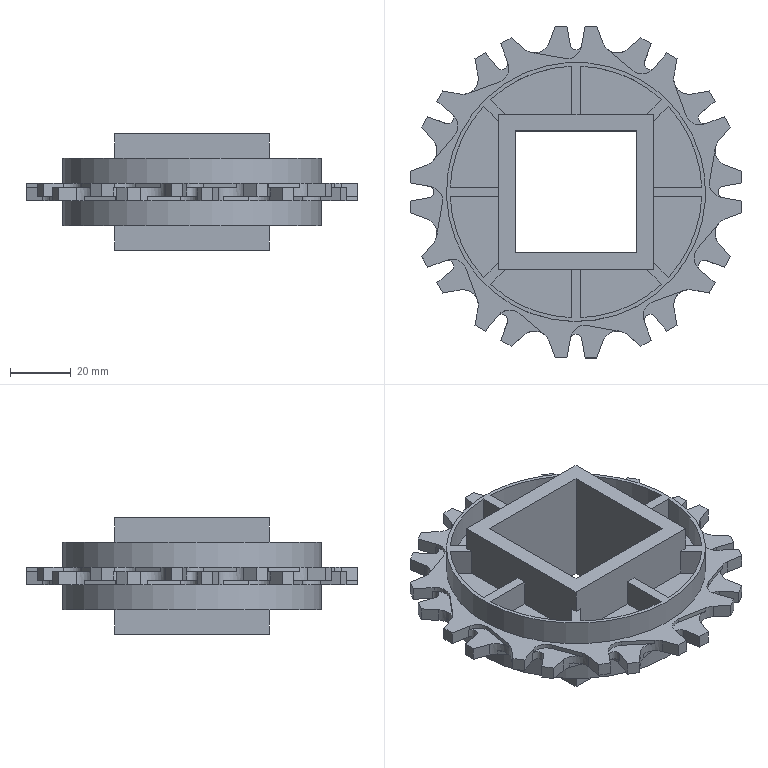Part | STEP file | s3d9xxcjk1ng | 1 solid | 254 faces | box 108.897 x 108.897 x 38.1 mm | volume 73401 mm3 | plane 186 | cylinder 68 | commonest cylinder face diameters 9.55 x24 82.55 x16 3.81 x12 10.16 x12 85.002 x4